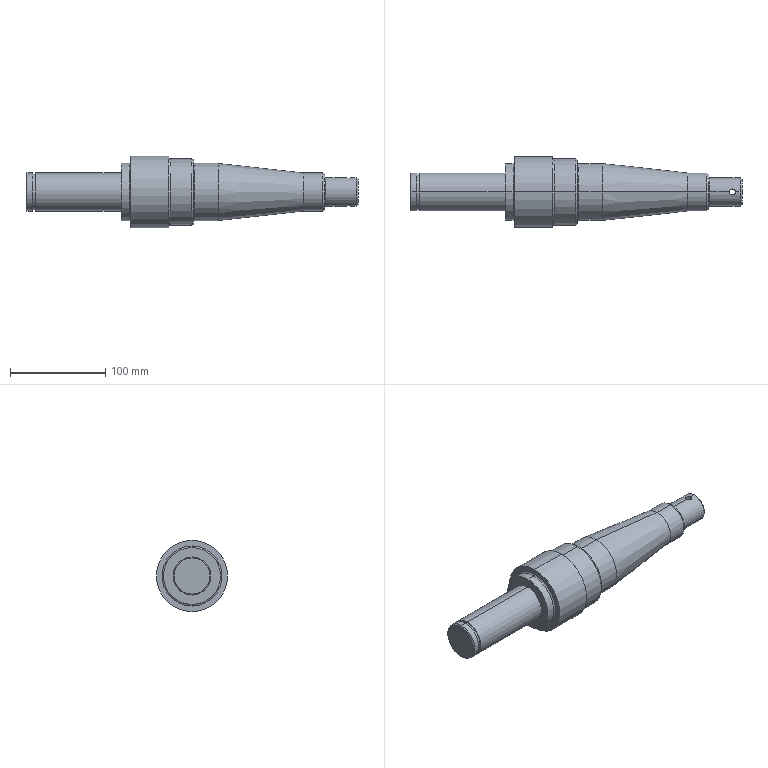Part | STEP file | SHAFT_AXIS_HOUSING1V11 | 1 solid | 47 faces | box 349 x 75 x 75 mm | volume 734000 mm3 | cylinder 20 | cone 10 | plane 9 | torus 8 | commonest cylinder face diameters 40 x6 60 x4 6.3 x2 30 x2 37.5 x2 70 x2